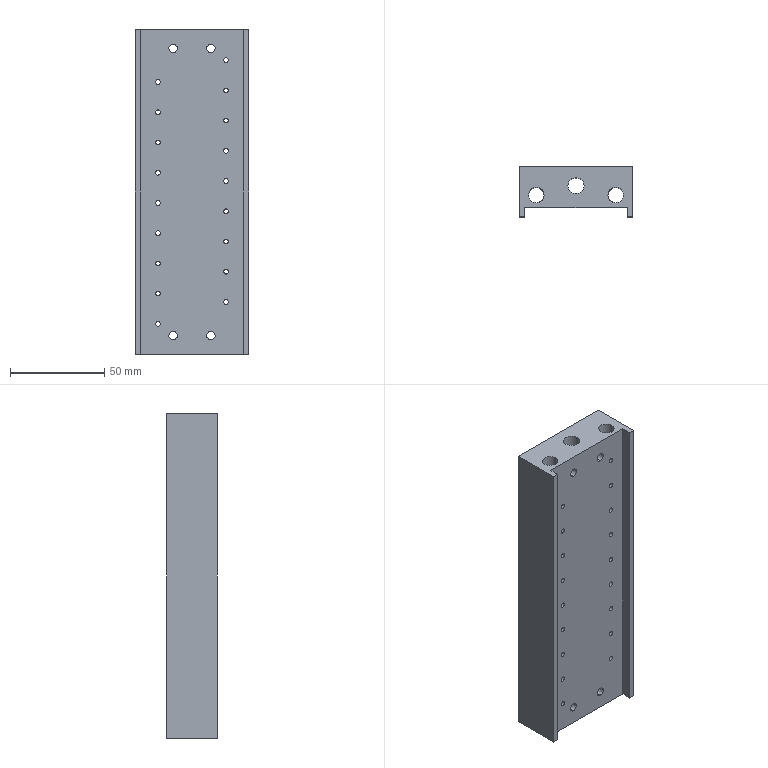Part | STEP file | 11-SS5Y5-20-09-V2.011 | 1 solid | 78 faces | box 60 x 26.5 x 172 mm | volume 195269 mm3 | cylinder 68 | plane 10 | commonest cylinder face diameters 2.5 x54 4.5 x8 8.162 x2 8.183 x2 8.573 x2